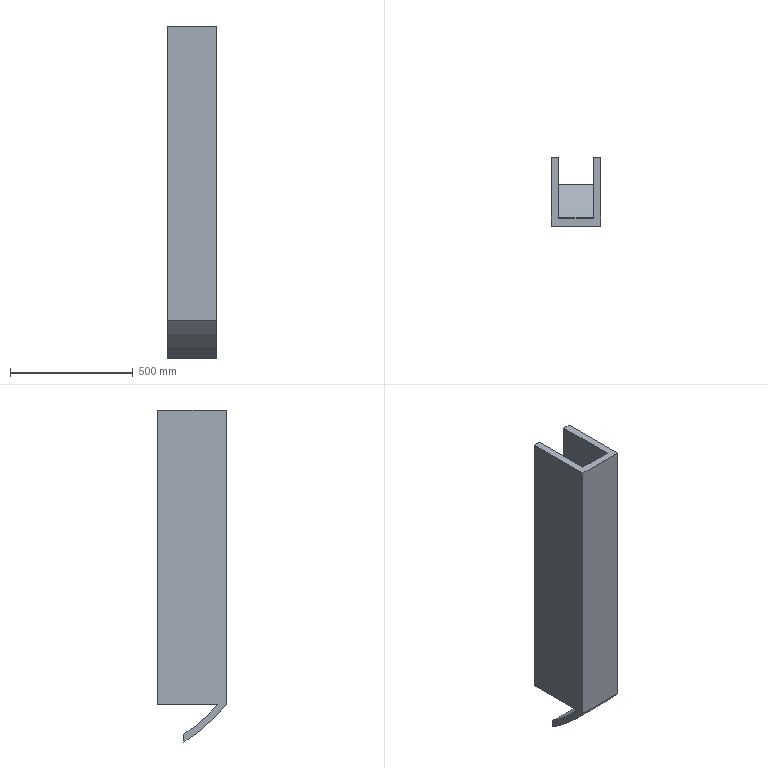Part | SolidWorks | features ICE 3, Extrusion 1 | 1 solid | 172 faces | box 200 x 280 x 1354 mm | volume 26886001 mm3 | plane 170 | cylinder 2 | commonest cylinder face diameters 1300 x1 1354 x1